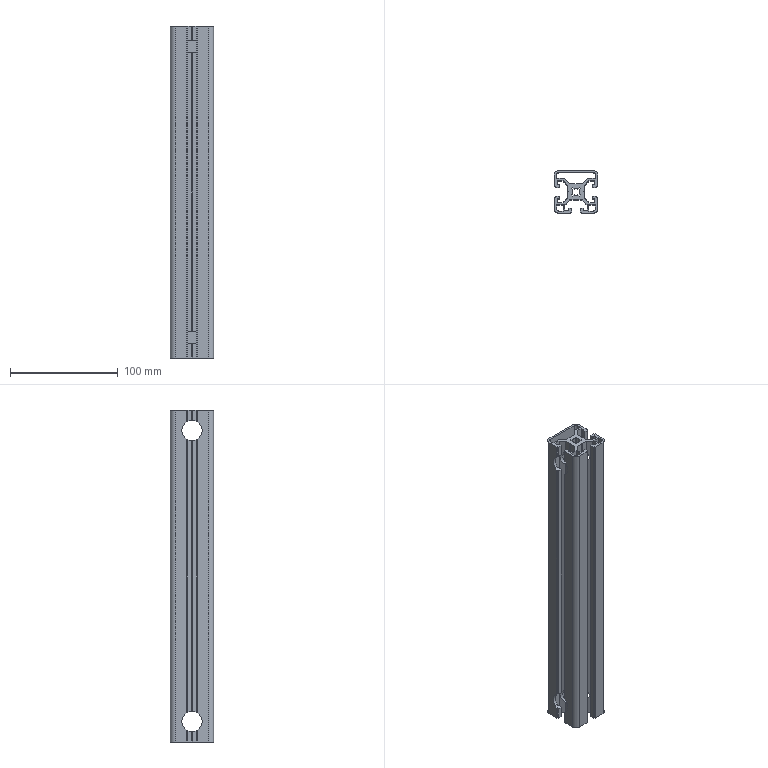Part | SolidWorks | features BaseBody 1, HoleWzd 1, MoveFace 1 | 1 solid | 242 faces | box 40 x 40 x 308 mm | volume 173974 mm3 | plane 187 | cylinder 55 | commonest cylinder face diameters 6.8 x15 2 x14 19 x12 1 x6 5 x4 9 x4